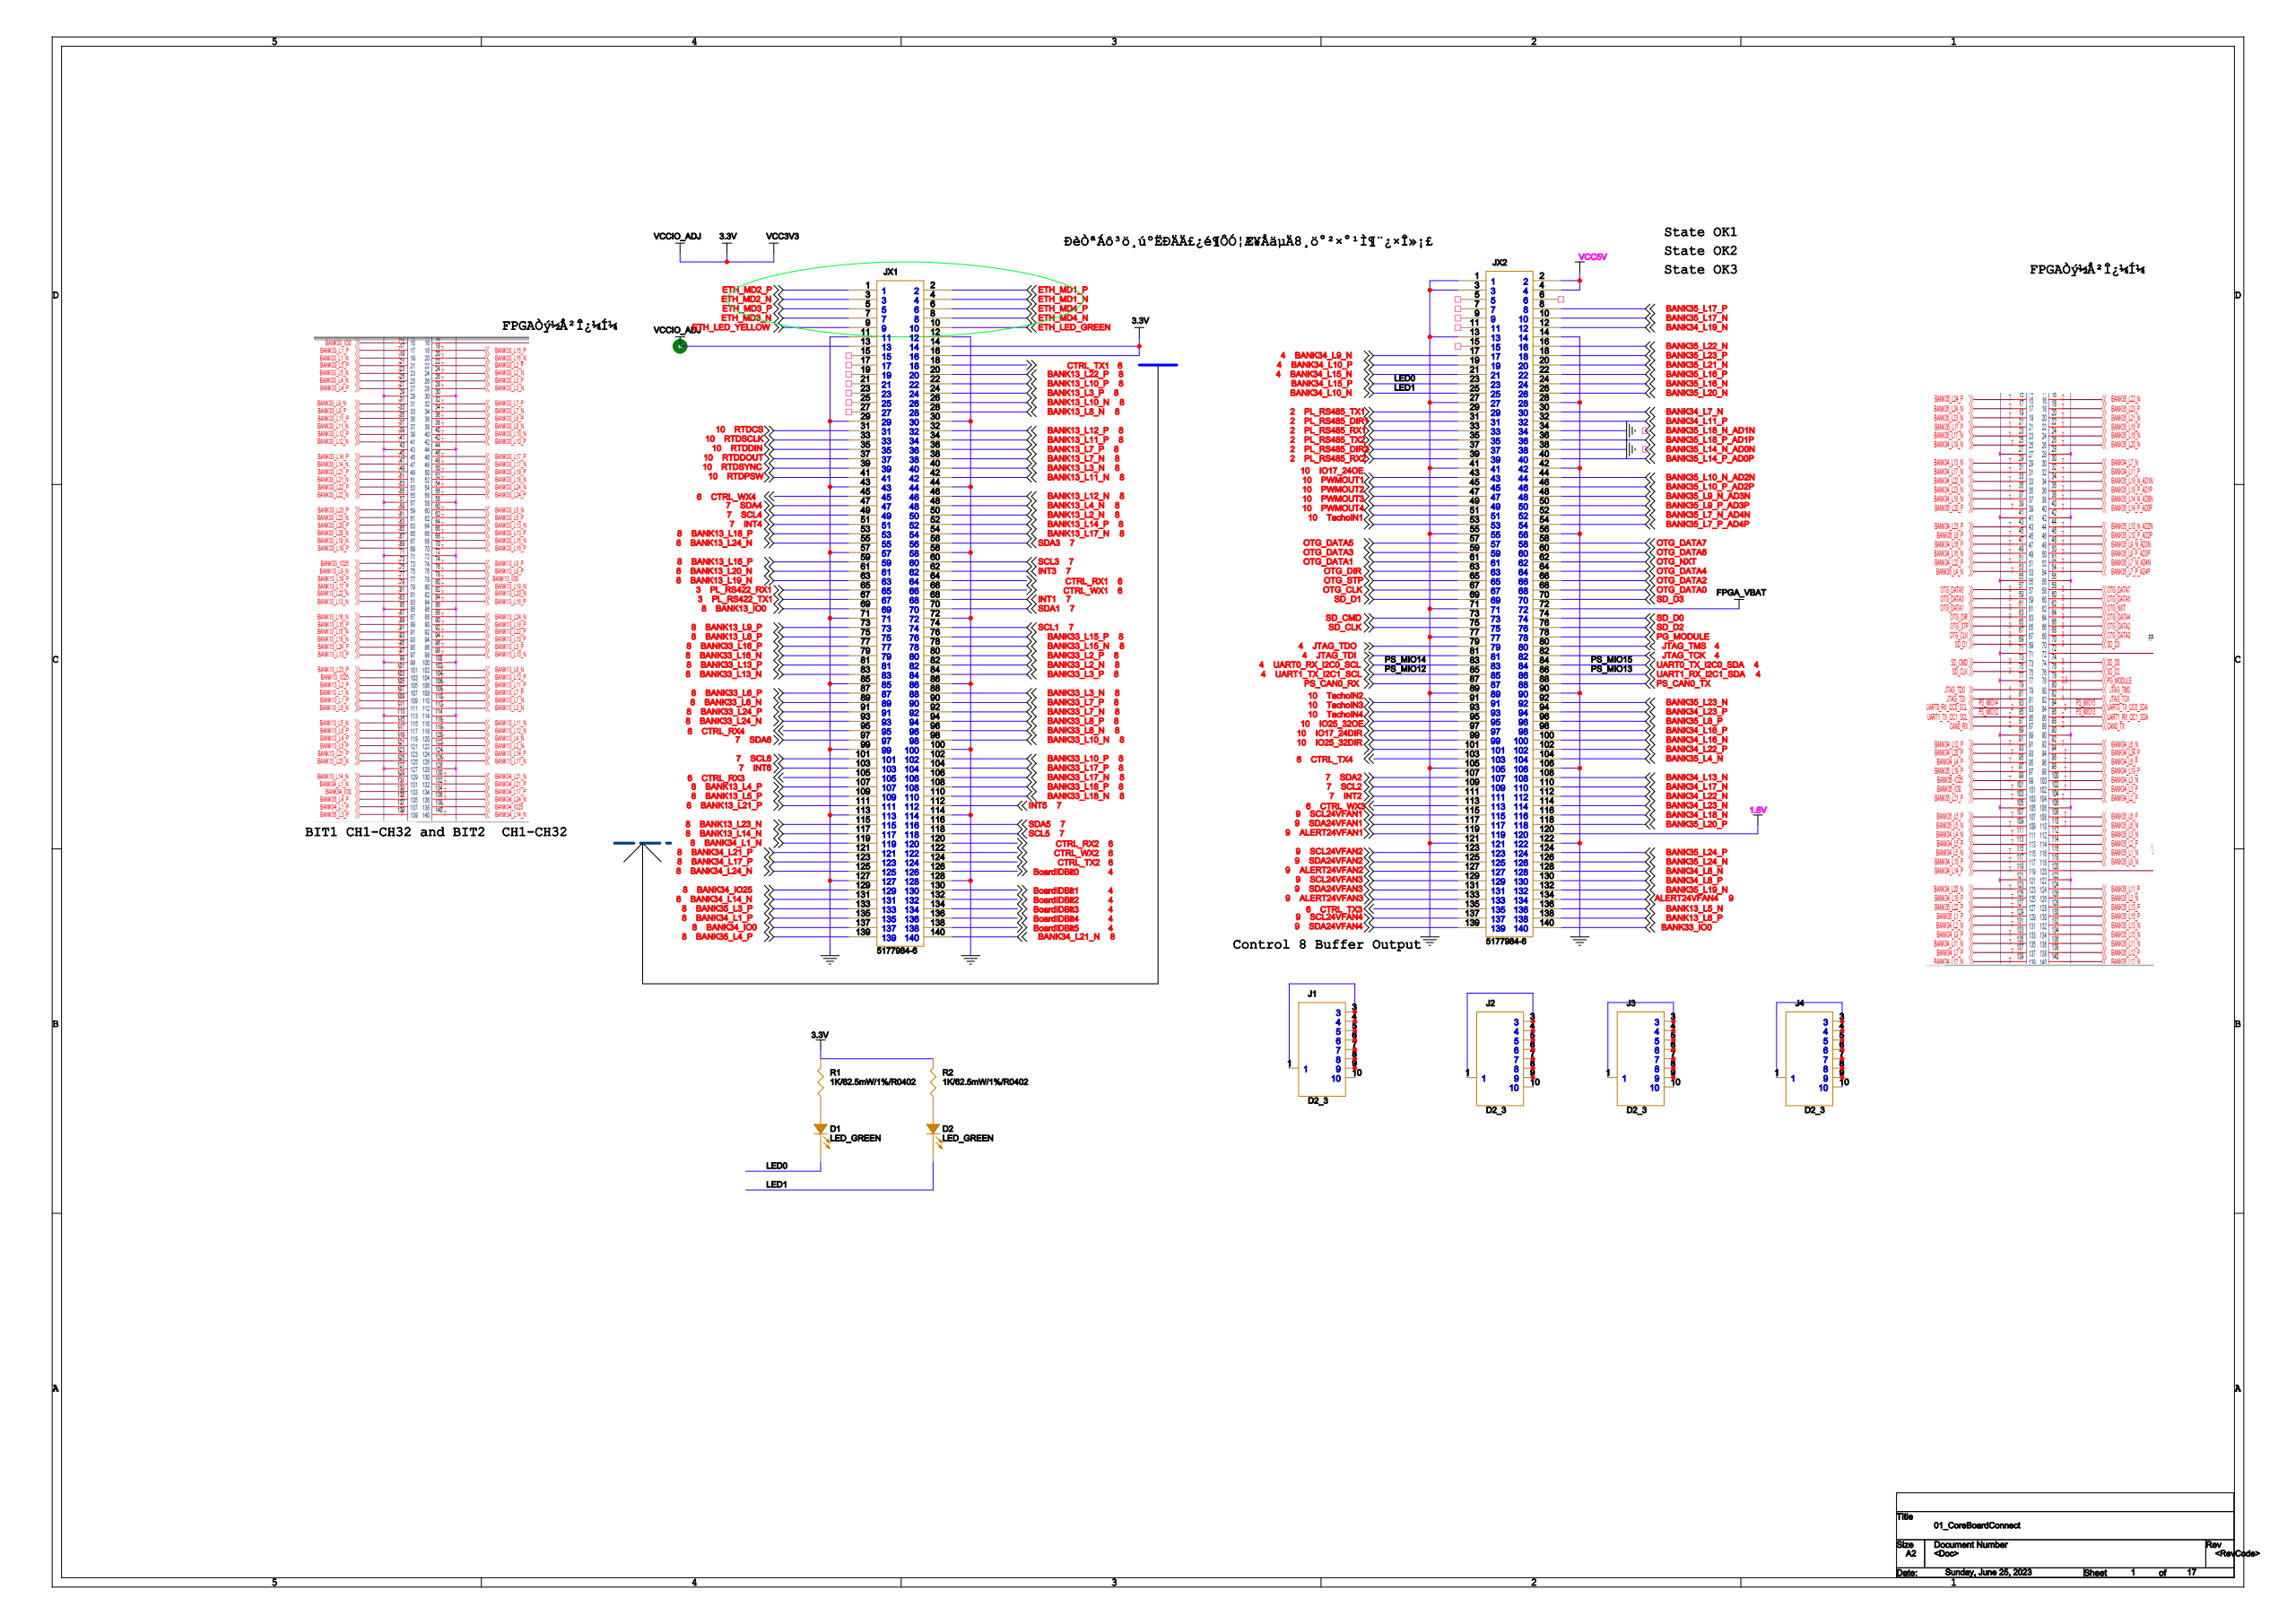Circuit board | Cadence Allegro | 1997 parts | 1536 nets | one sheet of the schematic
Parts on this sheet (reference | value | footprint):
D1 | LED_GREEN | LED0805
D2 | LED_GREEN | LED0805
J1 | D2_3 | D2_3
J2 | D2_3 | D2_3
J3 | D2_3 | D2_3
J4 | D2_3 | D2_3
JX1 | 5177984-6 | 5177983-6
JX2 | 5177984-6 | 5177983-6
R1 | 1K/62.5mW/1%/R0402 | 0402
R2 | 1K/62.5mW/1%/R0402 | 0402
Nets of these parts (net: part-pin ...):
3.3V: R1-2 R2-2 JX1-13 JX1-14 JX1-16
ETH_MD2_P: JX1-1
ETH_LED_GREEN: JX1-10
SCL6: JX1-101
BANK33_L10_P: JX1-102
INT6: JX1-103
BANK33_L17_P: JX1-104
CTRL_RX3: JX1-105
BANK33_L17_N: JX1-106
BANK13_L4_P: JX1-107
BANK33_L18_P: JX1-108
BANK13_L5_P: JX1-109
BANK33_L18_N: JX1-110
BANK13_L21_P: JX1-111
INT5: JX1-112
BANK13_L23_N: JX1-115
SDA5: JX1-116
BANK13_L14_N: JX1-117
SCL5: JX1-118
BANK34_L1_N: JX1-119
CTRL_RX2: JX1-120
BANK34_L21_P: JX1-121
CTRL_WX2: JX1-122
BANK34_L17_P: JX1-123
CTRL_TX2: JX1-124
BANK34_L24_N: JX1-125
BANK34_IO25: JX1-129
BANK34_L14_N: JX1-131
BANK35_L3_P: JX1-133
BANK34_L1_P: JX1-135
BANK34_IO0: JX1-137
BANK35_L4_P: JX1-139
BANK34_L21_N: JX1-140
CTRL_TX1: JX1-18
ETH_MD1_P: JX1-2
BANK13_L22_P: JX1-20
BANK13_L10_P: JX1-22
BANK13_L3_P: JX1-24
BANK13_L10_N: JX1-26
BANK13_L8_N: JX1-28
ETH_MD2_N: JX1-3
RTDCS: JX1-31
BANK13_L12_P: JX1-32
RTDSCLK: JX1-33
BANK13_L11_P: JX1-34
RTDDIN: JX1-35
BANK13_L7_P: JX1-36
RTDDOUT: JX1-37
BANK13_L7_N: JX1-38
RTDSYNC: JX1-39
ETH_MD1_N: JX1-4
BANK13_L3_N: JX1-40
RTDPSW: JX1-41
BANK13_L11_N: JX1-42
CTRL_WX4: JX1-45
BANK13_L12_N: JX1-46
SDA4: JX1-47
BANK13_L4_N: JX1-48
SCL4: JX1-49
ETH_MD3_P: JX1-5
BANK13_L2_N: JX1-50
INT4: JX1-51
BANK13_L14_P: JX1-52
BANK13_L18_P: JX1-53
BANK13_L17_N: JX1-54
BANK13_L24_N: JX1-55
SDA3: JX1-56
BANK13_L16_P: JX1-59
ETH_MD4_P: JX1-6
SCL3: JX1-60
BANK13_L20_N: JX1-61
INT3: JX1-62
BANK13_L19_N: JX1-63
CTRL_RX1: JX1-64
PL_RS422_RX1: JX1-65
CTRL_WX1: JX1-66
PL_RS422_TX1: JX1-67
INT1: JX1-68
BANK13_IO0: JX1-69
ETH_MD3_N: JX1-7
SDA1: JX1-70
BANK13_L9_P: JX1-73
SCL1: JX1-74
BANK13_L8_P: JX1-75
BANK33_L15_P: JX1-76
BANK33_L16_P: JX1-77
BANK33_L15_N: JX1-78
BANK33_L16_N: JX1-79
ETH_MD4_N: JX1-8
BANK33_L2_P: JX1-80
BANK33_L13_P: JX1-81
BANK33_L2_N: JX1-82
BANK33_L13_N: JX1-83
BANK33_L3_P: JX1-84
BANK33_L6_P: JX1-87
BANK33_L3_N: JX1-88
BANK33_L6_N: JX1-89
ETH_LED_YELLOW: JX1-9
BANK33_L7_P: JX1-90
BANK33_L24_P: JX1-91
BANK33_L7_N: JX1-92
BANK33_L24_N: JX1-93
BANK33_L8_P: JX1-94
CTRL_RX4: JX1-95
BANK33_L8_N: JX1-96
SDA6: JX1-97
BANK33_L10_N: JX1-98
BANK35_L17_N: JX2-10
BANK34_L16_N: JX2-100
IO25_32DIR: JX2-101
BANK34_L22_P: JX2-102
CTRL_TX4: JX2-103
BANK35_L4_N: JX2-104
SDA2: JX2-107
BANK34_L13_N: JX2-108
SCL2: JX2-109
BANK34_L17_N: JX2-110
INT2: JX2-111
BANK34_L22_N: JX2-112
CTRL_WX3: JX2-113
BANK34_L23_N: JX2-114
SCL24VFAN1: JX2-115
BANK34_L18_N: JX2-116
SDA24VFAN1: JX2-117
BANK35_L20_P: JX2-118
ALERT24VFAN1: JX2-119
BANK34_L19_N: JX2-12
1.8V: JX2-120
SCL24VFAN2: JX2-123
BANK35_L24_P: JX2-124
SDA24VFAN2: JX2-125
BANK35_L24_N: JX2-126
ALERT24VFAN2: JX2-127
BANK34_L8_N: JX2-128
SCL24VFAN3: JX2-129
BANK34_L8_P: JX2-130
SDA24VFAN3: JX2-131
BANK35_L19_N: JX2-132
ALERT24VFAN3: JX2-133
ALERT24VFAN4: JX2-134
CTRL_TX3: JX2-135
BANK13_L5_N: JX2-136
SCL24VFAN4: JX2-137
BANK13_L6_P: JX2-138
SDA24VFAN4: JX2-139
BANK33_IO0: JX2-140
BANK35_L22_N: JX2-16
BANK34_L9_N: JX2-17
BANK35_L23_P: JX2-18
BANK34_L10_P: JX2-19
VCC5V: JX2-2 JX2-4
BANK35_L21_N: JX2-20
BANK34_L15_N: JX2-21
BANK35_L16_P: JX2-22
BANK34_L15_P: D1-2 JX2-23
BANK35_L16_N: JX2-24
BANK34_L10_N: D2-2 JX2-25
BANK35_L20_N: JX2-26
PL_RS485_TX1: JX2-29
BANK34_L7_N: JX2-30
PL_RS485_DIR1: JX2-31
BANK34_L11_P: JX2-32
PL_RS485_RX1: JX2-33
PL_RS485_TX2: JX2-35
BANK35_L18_P_AD1P: JX2-36
PL_RS485_DIR2: JX2-37
PL_RS485_RX2: JX2-39
BANK35_L14_P_AD0P: JX2-40
IO17_24OE: JX2-43
BANK35_L10_N_AD2N: JX2-44
PWMOUT1: JX2-45
BANK35_L10_P_AD2P: JX2-46
PWMOUT2: JX2-47
BANK35_L9_N_AD3N: JX2-48
PWMOUT3: JX2-49
BANK35_L9_P_AD3P: JX2-50
PWMOUT4: JX2-51
BANK35_L7_N_AD4N: JX2-52
BANK35_L7_P_AD4P: JX2-54
OTG_DATA5: JX2-57
OTG_DATA7: JX2-58
OTG_DATA3: JX2-59
OTG_DATA6: JX2-60
OTG_DATA1: JX2-61
OTG_NXT: JX2-62
OTG_DIR: JX2-63
OTG_DATA4: JX2-64
OTG_STP: JX2-65
OTG_DATA2: JX2-66
OTG_CLK: JX2-67
OTG_DATA0: JX2-68
SD_D1: JX2-69
SD_D3: JX2-70
FPGA_VBAT: JX2-72
SD_CMD: JX2-73
SD_D0: JX2-74
SD_CLK: JX2-75
SD_D2: JX2-76
PG_MODULE: JX2-78
JTAG_TDO: JX2-79
BANK35_L17_P: JX2-8
JTAG_TMS: JX2-80
JTAG_TDI: JX2-81
JTAG_TCK: JX2-82
UART0_RX_I2C0_SCL: JX2-83
UART0_TX_I2C0_SDA: JX2-84
UART1_TX_I2C1_SCL: JX2-85
UART1_RX_I2C1_SDA: JX2-86
PS_CAN0_RX: JX2-87
PS_CAN0_TX: JX2-88
BANK35_L23_N: JX2-92
BANK34_L23_P: JX2-94
BANK35_L8_P: JX2-96
IO25_32OE: JX2-97
BANK34_L16_P: JX2-98
IO17_24DIR: JX2-99
N231084320: D1-1 R1-1
N231087860: D2-1 R2-1
N23884939: J1-1 J1-3 J1-4 J1-5 J1-6 J1-7 J1-8 J1-9 J1-10
N23884945: J2-1 J2-3 J2-4 J2-5 J2-6 J2-7 J2-8 J2-9 J2-10
N23884981: J3-1 J3-3 J3-4 J3-5 J3-6 J3-7 J3-8 J3-9 J3-10
N23884987: J4-1 J4-3 J4-4 J4-5 J4-6 J4-7 J4-8 J4-9 J4-10